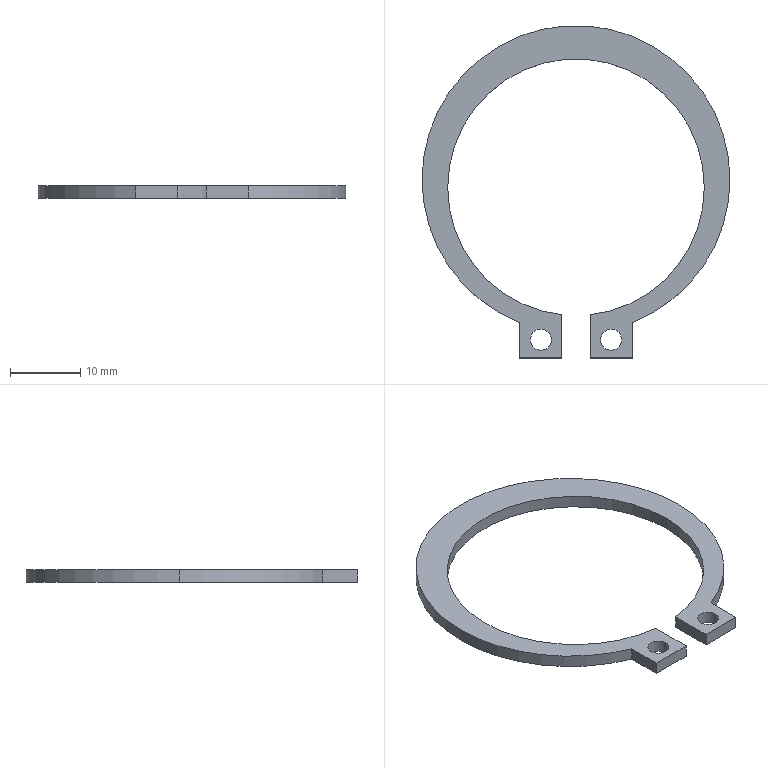Part | STEP file | Mkt stator clip | 1 solid | 18 faces | box 43.8 x 47.287 x 1.8 mm | volume 874.267 mm3 | cylinder 10 | plane 8 | commonest cylinder face diameters 3 x4 36.5 x3 43.8 x3
STEP:
#1=CARTESIAN_POINT('',(0.,0.,0.));
#2=DIRECTION('',(0.,0.,1.));
#3=DIRECTION('',(1.,0.,0.));
#4=AXIS2_PLACEMENT_3D('',#1,#2,#3);
#5=CARTESIAN_POINT('',(3.5,-21.7,1.8));
#6=VERTEX_POINT('',#5);
#7=CARTESIAN_POINT('',(3.5,-21.7,0.));
#8=VERTEX_POINT('',#7);
#9=CARTESIAN_POINT('',(3.5,-21.7,1.8));
#10=DIRECTION('',(0.,0.,-1.));
#11=VECTOR('',#10,1.);
#12=LINE('',#9,#11);
#13=CARTESIAN_POINT('',(5.,-21.7,1.8));
#14=DIRECTION('',(0.,0.,-1.));
#15=DIRECTION('',(-1.,0.,0.));
#16=AXIS2_PLACEMENT_3D('',#13,#14,#15);
#17=CYLINDRICAL_SURFACE('',#16,1.5);
#18=CARTESIAN_POINT('',(6.283,0.));
#19=DIRECTION('',(0.,1.));
#20=VECTOR('',#19,1.);
#21=LINE('',#18,#20);
#22=(GEOMETRIC_REPRESENTATION_CONTEXT(2)PARAMETRIC_REPRESENTATION_CONTEXT()REPRESENTATION_CONTEXT('',''));
#23=DEFINITIONAL_REPRESENTATION('',(#21),#22);
#24=PCURVE('',#17,#23);
#25=CARTESIAN_POINT('',(5.,-21.7,1.8));
#26=DIRECTION('',(0.,0.,-1.));
#27=DIRECTION('',(-1.,0.,0.));
#28=AXIS2_PLACEMENT_3D('',#25,#26,#27);
#29=CYLINDRICAL_SURFACE('',#28,1.5);
#30=CARTESIAN_POINT('',(0.,0.));
#31=DIRECTION('',(0.,1.));
#32=VECTOR('',#31,1.);
#33=LINE('',#30,#32);
#34=(GEOMETRIC_REPRESENTATION_CONTEXT(2)PARAMETRIC_REPRESENTATION_CONTEXT()REPRESENTATION_CONTEXT('',''));
#35=DEFINITIONAL_REPRESENTATION('',(#33),#34);
#36=PCURVE('',#29,#35);
#37=SURFACE_CURVE('',#12,(#24,#36),.PCURVE_S1.);
#38=EDGE_CURVE('',#6,#8,#37,.T.);
#39=ORIENTED_EDGE('',*,*,#38,.T.);
#40=CARTESIAN_POINT('',(6.5,-21.7,0.));
#41=VERTEX_POINT('',#40);
#42=CARTESIAN_POINT('',(5.,-21.7,0.));
#43=DIRECTION('',(0.,0.,1.));
#44=DIRECTION('',(-1.,0.,0.));
#45=AXIS2_PLACEMENT_3D('',#42,#43,#44);
#46=CIRCLE('',#45,1.5);
#47=CARTESIAN_POINT('',(6.283,1.8));
#48=DIRECTION('',(-1.,0.));
#49=VECTOR('',#48,1.);
#50=LINE('',#47,#49);
#51=(GEOMETRIC_REPRESENTATION_CONTEXT(2)PARAMETRIC_REPRESENTATION_CONTEXT()REPRESENTATION_CONTEXT('',''));
#52=DEFINITIONAL_REPRESENTATION('',(#50),#51);
#53=PCURVE('',#17,#52);
#54=CARTESIAN_POINT('',(0.,0.,0.));
#55=DIRECTION('',(0.,0.,1.));
#56=DIRECTION('',(1.,0.,0.));
#57=AXIS2_PLACEMENT_3D('',#54,#55,#56);
#58=PLANE('',#57);
#59=CARTESIAN_POINT('',(5.,-21.7));
#60=DIRECTION('',(-1.,0.));
#61=AXIS2_PLACEMENT_2D('',#59,#60);
#62=CIRCLE('',#61,1.5);
#63=(GEOMETRIC_REPRESENTATION_CONTEXT(2)PARAMETRIC_REPRESENTATION_CONTEXT()REPRESENTATION_CONTEXT('',''));
#64=DEFINITIONAL_REPRESENTATION('',(#62),#63);
#65=PCURVE('',#58,#64);
#66=SURFACE_CURVE('',#46,(#53,#65),.PCURVE_S1.);
#67=EDGE_CURVE('',#8,#41,#66,.T.);
#68=ORIENTED_EDGE('',*,*,#67,.T.);
#69=CARTESIAN_POINT('',(6.5,-21.7,1.8));
#70=VERTEX_POINT('',#69);
#71=CARTESIAN_POINT('',(6.5,-21.7,1.8));
#72=DIRECTION('',(0.,0.,-1.));
#73=VECTOR('',#72,1.);
#74=LINE('',#71,#73);
#75=CARTESIAN_POINT('',(3.142,0.));
#76=DIRECTION('',(0.,1.));
#77=VECTOR('',#76,1.);
#78=LINE('',#75,#77);
#79=(GEOMETRIC_REPRESENTATION_CONTEXT(2)PARAMETRIC_REPRESENTATION_CONTEXT()REPRESENTATION_CONTEXT('',''));
#80=DEFINITIONAL_REPRESENTATION('',(#78),#79);
#81=PCURVE('',#17,#80);
#82=CARTESIAN_POINT('',(3.142,0.));
#83=DIRECTION('',(0.,1.));
#84=VECTOR('',#83,1.);
#85=LINE('',#82,#84);
#86=(GEOMETRIC_REPRESENTATION_CONTEXT(2)PARAMETRIC_REPRESENTATION_CONTEXT()REPRESENTATION_CONTEXT('',''));
#87=DEFINITIONAL_REPRESENTATION('',(#85),#86);
#88=PCURVE('',#29,#87);
#89=SURFACE_CURVE('',#74,(#81,#88),.PCURVE_S1.);
#90=EDGE_CURVE('',#70,#41,#89,.T.);
#91=ORIENTED_EDGE('',*,*,#90,.F.);
#92=CARTESIAN_POINT('',(5.,-21.7,1.8));
#93=DIRECTION('',(0.,0.,-1.));
#94=DIRECTION('',(-1.,0.,0.));
#95=AXIS2_PLACEMENT_3D('',#92,#93,#94);
#96=CIRCLE('',#95,1.5);
#97=CARTESIAN_POINT('',(0.,0.));
#98=DIRECTION('',(1.,0.));
#99=VECTOR('',#98,1.);
#100=LINE('',#97,#99);
#101=(GEOMETRIC_REPRESENTATION_CONTEXT(2)PARAMETRIC_REPRESENTATION_CONTEXT()REPRESENTATION_CONTEXT('',''));
#102=DEFINITIONAL_REPRESENTATION('',(#100),#101);
#103=PCURVE('',#17,#102);
#104=CARTESIAN_POINT('',(0.,0.,1.8));
#105=DIRECTION('',(0.,0.,1.));
#106=DIRECTION('',(1.,0.,0.));
#107=AXIS2_PLACEMENT_3D('',#104,#105,#106);
#108=PLANE('',#107);
#109=CARTESIAN_POINT('',(3.5,-21.7));
#110=CARTESIAN_POINT('',(3.5,-19.102));
#111=CARTESIAN_POINT('',(5.75,-20.401));
#112=CARTESIAN_POINT('',(8.,-21.7));
#113=CARTESIAN_POINT('',(5.75,-22.999));
#114=CARTESIAN_POINT('',(3.5,-24.298));
#115=CARTESIAN_POINT('',(3.5,-21.7));
#116=(BOUNDED_CURVE()B_SPLINE_CURVE(2,(#109,#110,#111,#112,#113,#114,#115),.UNSPECIFIED.,.T.,.F.)B_SPLINE_CURVE_WITH_KNOTS((1,2,2,2,2,1),(-2.094,0.,2.094,4.189,6.283,8.378),.UNSPECIFIED.)CURVE()GEOMETRIC_REPRESENTATION_ITEM()RATIONAL_B_SPLINE_CURVE((1.,0.5,1.,0.5,1.,0.5,1.))REPRESENTATION_ITEM(''));
#117=(GEOMETRIC_REPRESENTATION_CONTEXT(2)PARAMETRIC_REPRESENTATION_CONTEXT()REPRESENTATION_CONTEXT('',''));
#118=DEFINITIONAL_REPRESENTATION('',(#116),#117);
#119=PCURVE('',#108,#118);
#120=SURFACE_CURVE('',#96,(#103,#119),.PCURVE_S1.);
#121=EDGE_CURVE('',#70,#6,#120,.T.);
#122=ORIENTED_EDGE('',*,*,#121,.T.);
#123=EDGE_LOOP('',(#39,#68,#91,#122));
#124=FACE_BOUND('',#123,.F.);
#125=ADVANCED_FACE('',(#124),#17,.F.);
#126=CARTESIAN_POINT('',(21.9,1.1,1.8));
#127=VERTEX_POINT('',#126);
#128=CARTESIAN_POINT('',(-21.9,1.1,1.8));
#129=VERTEX_POINT('',#128);
#130=CARTESIAN_POINT('',(0.,1.1,1.8));
#131=DIRECTION('',(0.,0.,1.));
#132=DIRECTION('',(-1.,0.,0.));
#133=AXIS2_PLACEMENT_3D('',#130,#131,#132);
#134=CIRCLE('',#133,21.9);
#135=CARTESIAN_POINT('',(0.,1.1,1.8));
#136=DIRECTION('',(0.,0.,-1.));
#137=DIRECTION('',(-1.,0.,0.));
#138=AXIS2_PLACEMENT_3D('',#135,#136,#137);
#139=CYLINDRICAL_SURFACE('',#138,21.9);
#140=CARTESIAN_POINT('',(6.283,0.));
#141=DIRECTION('',(-1.,0.));
#142=VECTOR('',#141,1.);
#143=LINE('',#140,#142);
#144=(GEOMETRIC_REPRESENTATION_CONTEXT(2)PARAMETRIC_REPRESENTATION_CONTEXT()REPRESENTATION_CONTEXT('',''));
#145=DEFINITIONAL_REPRESENTATION('',(#143),#144);
#146=PCURVE('',#139,#145);
#147=CARTESIAN_POINT('',(0.,1.1));
#148=DIRECTION('',(-1.,0.));
#149=AXIS2_PLACEMENT_2D('',#147,#148);
#150=CIRCLE('',#149,21.9);
#151=(GEOMETRIC_REPRESENTATION_CONTEXT(2)PARAMETRIC_REPRESENTATION_CONTEXT()REPRESENTATION_CONTEXT('',''));
#152=DEFINITIONAL_REPRESENTATION('',(#150),#151);
#153=PCURVE('',#108,#152);
#154=SURFACE_CURVE('',#134,(#146,#153),.PCURVE_S1.);
#155=EDGE_CURVE('',#127,#129,#154,.T.);
#156=ORIENTED_EDGE('',*,*,#155,.F.);
#157=CARTESIAN_POINT('',(21.9,1.1,0.));
#158=VERTEX_POINT('',#157);
#159=CARTESIAN_POINT('',(21.9,1.1,1.8));
#160=DIRECTION('',(0.,0.,-1.));
#161=VECTOR('',#160,1.);
#162=LINE('',#159,#161);
#163=CARTESIAN_POINT('',(3.142,0.));
#164=DIRECTION('',(0.,1.));
#165=VECTOR('',#164,1.);
#166=LINE('',#163,#165);
#167=(GEOMETRIC_REPRESENTATION_CONTEXT(2)PARAMETRIC_REPRESENTATION_CONTEXT()REPRESENTATION_CONTEXT('',''));
#168=DEFINITIONAL_REPRESENTATION('',(#166),#167);
#169=PCURVE('',#139,#168);
#170=CARTESIAN_POINT('',(0.,1.1,1.8));
#171=DIRECTION('',(0.,0.,-1.));
#172=DIRECTION('',(-1.,0.,0.));
#173=AXIS2_PLACEMENT_3D('',#170,#171,#172);
#174=CYLINDRICAL_SURFACE('',#173,21.9);
#175=CARTESIAN_POINT('',(3.142,0.));
#176=DIRECTION('',(0.,1.));
#177=VECTOR('',#176,1.);
#178=LINE('',#175,#177);
#179=(GEOMETRIC_REPRESENTATION_CONTEXT(2)PARAMETRIC_REPRESENTATION_CONTEXT()REPRESENTATION_CONTEXT('',''));
#180=DEFINITIONAL_REPRESENTATION('',(#178),#179);
#181=PCURVE('',#174,#180);
#182=SURFACE_CURVE('',#162,(#169,#181),.PCURVE_S1.);
#183=EDGE_CURVE('',#127,#158,#182,.T.);
#184=ORIENTED_EDGE('',*,*,#183,.T.);
#185=CARTESIAN_POINT('',(-21.9,1.1,0.));
#186=VERTEX_POINT('',#185);
#187=CARTESIAN_POINT('',(0.,1.1,0.));
#188=DIRECTION('',(0.,0.,1.));
#189=DIRECTION('',(-1.,0.,0.));
#190=AXIS2_PLACEMENT_3D('',#187,#188,#189);
#191=CIRCLE('',#190,21.9);
#192=CARTESIAN_POINT('',(6.283,1.8));
#193=DIRECTION('',(-1.,0.));
#194=VECTOR('',#193,1.);
#195=LINE('',#192,#194);
#196=(GEOMETRIC_REPRESENTATION_CONTEXT(2)PARAMETRIC_REPRESENTATION_CONTEXT()REPRESENTATION_CONTEXT('',''));
#197=DEFINITIONAL_REPRESENTATION('',(#195),#196);
#198=PCURVE('',#139,#197);
#199=CARTESIAN_POINT('',(0.,1.1));
#200=DIRECTION('',(-1.,0.));
#201=AXIS2_PLACEMENT_2D('',#199,#200);
#202=CIRCLE('',#201,21.9);
#203=(GEOMETRIC_REPRESENTATION_CONTEXT(2)PARAMETRIC_REPRESENTATION_CONTEXT()REPRESENTATION_CONTEXT('',''));
#204=DEFINITIONAL_REPRESENTATION('',(#202),#203);
#205=PCURVE('',#58,#204);
#206=SURFACE_CURVE('',#191,(#198,#205),.PCURVE_S1.);
#207=EDGE_CURVE('',#158,#186,#206,.T.);
#208=ORIENTED_EDGE('',*,*,#207,.T.);
#209=CARTESIAN_POINT('',(-21.9,1.1,1.8));
#210=DIRECTION('',(0.,0.,-1.));
#211=VECTOR('',#210,1.);
#212=LINE('',#209,#211);
#213=CARTESIAN_POINT('',(0.,0.));
#214=DIRECTION('',(0.,1.));
#215=VECTOR('',#214,1.);
#216=LINE('',#213,#215);
#217=(GEOMETRIC_REPRESENTATION_CONTEXT(2)PARAMETRIC_REPRESENTATION_CONTEXT()REPRESENTATION_CONTEXT('',''));
#218=DEFINITIONAL_REPRESENTATION('',(#216),#217);
#219=PCURVE('',#139,#218);
#220=CARTESIAN_POINT('',(0.,1.1,1.8));
#221=DIRECTION('',(0.,0.,-1.));
#222=DIRECTION('',(-1.,0.,0.));
#223=AXIS2_PLACEMENT_3D('',#220,#221,#222);
#224=CYLINDRICAL_SURFACE('',#223,21.9);
#225=CARTESIAN_POINT('',(6.283,0.));
#226=DIRECTION('',(0.,1.));
#227=VECTOR('',#226,1.);
#228=LINE('',#225,#227);
#229=(GEOMETRIC_REPRESENTATION_CONTEXT(2)PARAMETRIC_REPRESENTATION_CONTEXT()REPRESENTATION_CONTEXT('',''));
#230=DEFINITIONAL_REPRESENTATION('',(#228),#229);
#231=PCURVE('',#224,#230);
#232=SURFACE_CURVE('',#212,(#219,#231),.PCURVE_S1.);
#233=EDGE_CURVE('',#129,#186,#232,.T.);
#234=ORIENTED_EDGE('',*,*,#233,.F.);
#235=EDGE_LOOP('',(#156,#184,#208,#234));
#236=FACE_BOUND('',#235,.T.);
#237=ADVANCED_FACE('',(#236),#139,.T.);
#238=CARTESIAN_POINT('',(-8.,-19.287,1.8));
#239=VERTEX_POINT('',#238);
#240=CARTESIAN_POINT('',(0.,1.1,1.8));
#241=DIRECTION('',(0.,0.,1.));
#242=DIRECTION('',(-1.,0.,0.));
#243=AXIS2_PLACEMENT_3D('',#240,#241,#242);
#244=CIRCLE('',#243,21.9);
#245=CARTESIAN_POINT('',(6.283,0.));
#246=DIRECTION('',(-1.,0.));
#247=VECTOR('',#246,1.);
#248=LINE('',#245,#247);
#249=(GEOMETRIC_REPRESENTATION_CONTEXT(2)PARAMETRIC_REPRESENTATION_CONTEXT()REPRESENTATION_CONTEXT('',''));
#250=DEFINITIONAL_REPRESENTATION('',(#248),#249);
#251=PCURVE('',#224,#250);
#252=CARTESIAN_POINT('',(0.,1.1));
#253=DIRECTION('',(-1.,0.));
#254=AXIS2_PLACEMENT_2D('',#252,#253);
#255=CIRCLE('',#254,21.9);
#256=(GEOMETRIC_REPRESENTATION_CONTEXT(2)PARAMETRIC_REPRESENTATION_CONTEXT()REPRESENTATION_CONTEXT('',''));
#257=DEFINITIONAL_REPRESENTATION('',(#255),#256);
#258=PCURVE('',#108,#257);
#259=SURFACE_CURVE('',#244,(#251,#258),.PCURVE_S1.);
#260=EDGE_CURVE('',#129,#239,#259,.T.);
#261=ORIENTED_EDGE('',*,*,#260,.F.);
#262=ORIENTED_EDGE('',*,*,#233,.T.);
#263=CARTESIAN_POINT('',(-8.,-19.287,0.));
#264=VERTEX_POINT('',#263);
#265=CARTESIAN_POINT('',(0.,1.1,0.));
#266=DIRECTION('',(0.,0.,1.));
#267=DIRECTION('',(-1.,0.,0.));
#268=AXIS2_PLACEMENT_3D('',#265,#266,#267);
#269=CIRCLE('',#268,21.9);
#270=CARTESIAN_POINT('',(6.283,1.8));
#271=DIRECTION('',(-1.,0.));
#272=VECTOR('',#271,1.);
#273=LINE('',#270,#272);
#274=(GEOMETRIC_REPRESENTATION_CONTEXT(2)PARAMETRIC_REPRESENTATION_CONTEXT()REPRESENTATION_CONTEXT('',''));
#275=DEFINITIONAL_REPRESENTATION('',(#273),#274);
#276=PCURVE('',#224,#275);
#277=CARTESIAN_POINT('',(0.,1.1));
#278=DIRECTION('',(-1.,0.));
#279=AXIS2_PLACEMENT_2D('',#277,#278);
#280=CIRCLE('',#279,21.9);
#281=(GEOMETRIC_REPRESENTATION_CONTEXT(2)PARAMETRIC_REPRESENTATION_CONTEXT()REPRESENTATION_CONTEXT('',''));
#282=DEFINITIONAL_REPRESENTATION('',(#280),#281);
#283=PCURVE('',#58,#282);
#284=SURFACE_CURVE('',#269,(#276,#283),.PCURVE_S1.);
#285=EDGE_CURVE('',#186,#264,#284,.T.);
#286=ORIENTED_EDGE('',*,*,#285,.T.);
#287=CARTESIAN_POINT('',(-8.,-19.287,1.8));
#288=DIRECTION('',(0.,0.,1.));
#289=VECTOR('',#288,1.);
#290=LINE('',#287,#289);
#291=CARTESIAN_POINT('',(5.086,0.));
#292=DIRECTION('',(0.,-1.));
#293=VECTOR('',#292,1.);
#294=LINE('',#291,#293);
#295=(GEOMETRIC_REPRESENTATION_CONTEXT(2)PARAMETRIC_REPRESENTATION_CONTEXT()REPRESENTATION_CONTEXT('',''));
#296=DEFINITIONAL_REPRESENTATION('',(#294),#295);
#297=PCURVE('',#224,#296);
#298=CARTESIAN_POINT('',(-8.,-24.287,1.8));
#299=DIRECTION('',(1.,0.,0.));
#300=DIRECTION('',(0.,1.,0.));
#301=AXIS2_PLACEMENT_3D('',#298,#299,#300);
#302=PLANE('',#301);
#303=CARTESIAN_POINT('',(5.,0.));
#304=DIRECTION('',(0.,1.));
#305=VECTOR('',#304,1.);
#306=LINE('',#303,#305);
#307=(GEOMETRIC_REPRESENTATION_CONTEXT(2)PARAMETRIC_REPRESENTATION_CONTEXT()REPRESENTATION_CONTEXT('',''));
#308=DEFINITIONAL_REPRESENTATION('',(#306),#307);
#309=PCURVE('',#302,#308);
#310=SURFACE_CURVE('',#290,(#297,#309),.PCURVE_S1.);
#311=EDGE_CURVE('',#264,#239,#310,.T.);
#312=ORIENTED_EDGE('',*,*,#311,.T.);
#313=EDGE_LOOP('',(#261,#262,#286,#312));
#314=FACE_BOUND('',#313,.T.);
#315=ADVANCED_FACE('',(#314),#224,.T.);
#316=CARTESIAN_POINT('',(2.,-18.14,0.));
#317=VERTEX_POINT('',#316);
#318=CARTESIAN_POINT('',(2.,-18.14,1.8));
#319=VERTEX_POINT('',#318);
#320=CARTESIAN_POINT('',(2.,-18.14,1.8));
#321=DIRECTION('',(0.,0.,1.));
#322=VECTOR('',#321,1.);
#323=LINE('',#320,#322);
#324=CARTESIAN_POINT('',(0.,0.,1.8));
#325=DIRECTION('',(0.,0.,-1.));
#326=DIRECTION('',(-1.,0.,0.));
#327=AXIS2_PLACEMENT_3D('',#324,#325,#326);
#328=CYLINDRICAL_SURFACE('',#327,18.25);
#329=CARTESIAN_POINT('',(4.603,0.));
#330=DIRECTION('',(0.,-1.));
#331=VECTOR('',#330,1.);
#332=LINE('',#329,#331);
#333=(GEOMETRIC_REPRESENTATION_CONTEXT(2)PARAMETRIC_REPRESENTATION_CONTEXT()REPRESENTATION_CONTEXT('',''));
#334=DEFINITIONAL_REPRESENTATION('',(#332),#333);
#335=PCURVE('',#328,#334);
#336=CARTESIAN_POINT('',(2.,-24.287,1.8));
#337=DIRECTION('',(1.,0.,0.));
#338=DIRECTION('',(0.,1.,0.));
#339=AXIS2_PLACEMENT_3D('',#336,#337,#338);
#340=PLANE('',#339);
#341=CARTESIAN_POINT('',(6.146,0.));
#342=DIRECTION('',(0.,1.));
#343=VECTOR('',#342,1.);
#344=LINE('',#341,#343);
#345=(GEOMETRIC_REPRESENTATION_CONTEXT(2)PARAMETRIC_REPRESENTATION_CONTEXT()REPRESENTATION_CONTEXT('',''));
#346=DEFINITIONAL_REPRESENTATION('',(#344),#345);
#347=PCURVE('',#340,#346);
#348=SURFACE_CURVE('',#323,(#335,#347),.PCURVE_S1.);
#349=EDGE_CURVE('',#317,#319,#348,.T.);
#350=ORIENTED_EDGE('',*,*,#349,.F.);
#351=CARTESIAN_POINT('',(18.25,0.,0.));
#352=VERTEX_POINT('',#351);
#353=CARTESIAN_POINT('',(0.,0.,0.));
#354=DIRECTION('',(0.,0.,1.));
#355=DIRECTION('',(-1.,0.,0.));
#356=AXIS2_PLACEMENT_3D('',#353,#354,#355);
#357=CIRCLE('',#356,18.25);
#358=CARTESIAN_POINT('',(6.283,1.8));
#359=DIRECTION('',(-1.,0.));
#360=VECTOR('',#359,1.);
#361=LINE('',#358,#360);
#362=(GEOMETRIC_REPRESENTATION_CONTEXT(2)PARAMETRIC_REPRESENTATION_CONTEXT()REPRESENTATION_CONTEXT('',''));
#363=DEFINITIONAL_REPRESENTATION('',(#361),#362);
#364=PCURVE('',#328,#363);
#365=CARTESIAN_POINT('',(0.,0.));
#366=DIRECTION('',(-1.,0.));
#367=AXIS2_PLACEMENT_2D('',#365,#366);
#368=CIRCLE('',#367,18.25);
#369=(GEOMETRIC_REPRESENTATION_CONTEXT(2)PARAMETRIC_REPRESENTATION_CONTEXT()REPRESENTATION_CONTEXT('',''));
#370=DEFINITIONAL_REPRESENTATION('',(#368),#369);
#371=PCURVE('',#58,#370);
#372=SURFACE_CURVE('',#357,(#364,#371),.PCURVE_S1.);
#373=EDGE_CURVE('',#317,#352,#372,.T.);
#374=ORIENTED_EDGE('',*,*,#373,.T.);
#375=CARTESIAN_POINT('',(18.25,0.,1.8));
#376=VERTEX_POINT('',#375);
#377=CARTESIAN_POINT('',(18.25,0.,1.8));
#378=DIRECTION('',(0.,0.,-1.));
#379=VECTOR('',#378,1.);
#380=LINE('',#377,#379);
#381=CARTESIAN_POINT('',(3.142,0.));
#382=DIRECTION('',(0.,1.));
#383=VECTOR('',#382,1.);
#384=LINE('',#381,#383);
#385=(GEOMETRIC_REPRESENTATION_CONTEXT(2)PARAMETRIC_REPRESENTATION_CONTEXT()REPRESENTATION_CONTEXT('',''));
#386=DEFINITIONAL_REPRESENTATION('',(#384),#385);
#387=PCURVE('',#328,#386);
#388=CARTESIAN_POINT('',(0.,0.,1.8));
#389=DIRECTION('',(0.,0.,-1.));
#390=DIRECTION('',(-1.,0.,0.));
#391=AXIS2_PLACEMENT_3D('',#388,#389,#390);
#392=CYLINDRICAL_SURFACE('',#391,18.25);
#393=CARTESIAN_POINT('',(3.142,0.));
#394=DIRECTION('',(0.,1.));
#395=VECTOR('',#394,1.);
#396=LINE('',#393,#395);
#397=(GEOMETRIC_REPRESENTATION_CONTEXT(2)PARAMETRIC_REPRESENTATION_CONTEXT()REPRESENTATION_CONTEXT('',''));
#398=DEFINITIONAL_REPRESENTATION('',(#396),#397);
#399=PCURVE('',#392,#398);
#400=SURFACE_CURVE('',#380,(#387,#399),.PCURVE_S1.);
#401=EDGE_CURVE('',#376,#352,#400,.T.);
#402=ORIENTED_EDGE('',*,*,#401,.F.);
#403=CARTESIAN_POINT('',(0.,0.,1.8));
#404=DIRECTION('',(0.,0.,-1.));
#405=DIRECTION('',(-1.,0.,0.));
#406=AXIS2_PLACEMENT_3D('',#403,#404,#405);
#407=CIRCLE('',#406,18.25);
#408=CARTESIAN_POINT('',(0.,0.));
#409=DIRECTION('',(1.,0.));
#410=VECTOR('',#409,1.);
#411=LINE('',#408,#410);
#412=(GEOMETRIC_REPRESENTATION_CONTEXT(2)PARAMETRIC_REPRESENTATION_CONTEXT()REPRESENTATION_CONTEXT('',''));
#413=DEFINITIONAL_REPRESENTATION('',(#411),#412);
#414=PCURVE('',#328,#413);
#415=CARTESIAN_POINT('',(-18.25,0.));
#416=CARTESIAN_POINT('',(-18.25,31.61));
#417=CARTESIAN_POINT('',(9.125,15.805));
#418=CARTESIAN_POINT('',(36.5,0.));
#419=CARTESIAN_POINT('',(9.125,-15.805));
#420=CARTESIAN_POINT('',(-18.25,-31.61));
#421=CARTESIAN_POINT('',(-18.25,0.));
#422=(BOUNDED_CURVE()B_SPLINE_CURVE(2,(#415,#416,#417,#418,#419,#420,#421),.UNSPECIFIED.,.T.,.F.)B_SPLINE_CURVE_WITH_KNOTS((1,2,2,2,2,1),(-2.094,0.,2.094,4.189,6.283,8.378),.UNSPECIFIED.)CURVE()GEOMETRIC_REPRESENTATION_ITEM()RATIONAL_B_SPLINE_CURVE((1.,0.5,1.,0.5,1.,0.5,1.))REPRESENTATION_ITEM(''));
#423=(GEOMETRIC_REPRESENTATION_CONTEXT(2)PARAMETRIC_REPRESENTATION_CONTEXT()REPRESENTATION_CONTEXT('',''));
#424=DEFINITIONAL_REPRESENTATION('',(#422),#423);
#425=PCURVE('',#108,#424);
#426=SURFACE_CURVE('',#407,(#414,#425),.PCURVE_S1.);
#427=EDGE_CURVE('',#376,#319,#426,.T.);
#428=ORIENTED_EDGE('',*,*,#427,.T.);
#429=EDGE_LOOP('',(#350,#374,#402,#428));
#430=FACE_BOUND('',#429,.F.);
#431=ADVANCED_FACE('',(#430),#328,.F.);
#432=CARTESIAN_POINT('',(-18.25,0.,0.));
#433=VERTEX_POINT('',#432);
#434=CARTESIAN_POINT('',(0.,0.,0.));
#435=DIRECTION('',(0.,0.,1.));
#436=DIRECTION('',(-1.,0.,0.));
#437=AXIS2_PLACEMENT_3D('',#434,#435,#436);
#438=CIRCLE('',#437,18.25);
#439=CARTESIAN_POINT('',(6.283,1.8));
#440=DIRECTION('',(-1.,0.));
#441=VECTOR('',#440,1.);
#442=LINE('',#439,#441);
#443=(GEOMETRIC_REPRESENTATION_CONTEXT(2)PARAMETRIC_REPRESENTATION_CONTEXT()REPRESENTATION_CONTEXT('',''));
#444=DEFINITIONAL_REPRESENTATION('',(#442),#443);
#445=PCURVE('',#392,#444);
#446=CARTESIAN_POINT('',(0.,0.));
#447=DIRECTION('',(-1.,0.));
#448=AXIS2_PLACEMENT_2D('',#446,#447);
#449=CIRCLE('',#448,18.25);
#450=(GEOMETRIC_REPRESENTATION_CONTEXT(2)PARAMETRIC_REPRESENTATION_CONTEXT()REPRESENTATION_CONTEXT('',''));
#451=DEFINITIONAL_REPRESENTATION('',(#449),#450);
#452=PCURVE('',#58,#451);
#453=SURFACE_CURVE('',#438,(#445,#452),.PCURVE_S1.);
#454=EDGE_CURVE('',#352,#433,#453,.T.);
#455=ORIENTED_EDGE('',*,*,#454,.T.);
#456=CARTESIAN_POINT('',(-18.25,0.,1.8));
#457=VERTEX_POINT('',#456);
#458=CARTESIAN_POINT('',(-18.25,0.,1.8));
#459=DIRECTION('',(0.,0.,-1.));
#460=VECTOR('',#459,1.);
#461=LINE('',#458,#460);
#462=CARTESIAN_POINT('',(0.,0.));
#463=DIRECTION('',(0.,1.));
#464=VECTOR('',#463,1.);
#465=LINE('',#462,#464);
#466=(GEOMETRIC_REPRESENTATION_CONTEXT(2)PARAMETRIC_REPRESENTATION_CONTEXT()REPRESENTATION_CONTEXT('',''));
#467=DEFINITIONAL_REPRESENTATION('',(#465),#466);
#468=PCURVE('',#392,#467);
#469=CARTESIAN_POINT('',(0.,0.,1.8));
#470=DIRECTION('',(0.,0.,-1.));
#471=DIRECTION('',(-1.,0.,0.));
#472=AXIS2_PLACEMENT_3D('',#469,#470,#471);
#473=CYLINDRICAL_SURFACE('',#472,18.25);
#474=CARTESIAN_POINT('',(6.283,0.));
#475=DIRECTION('',(0.,1.));
#476=VECTOR('',#475,1.);
#477=LINE('',#474,#476);
#478=(GEOMETRIC_REPRESENTATION_CONTEXT(2)PARAMETRIC_REPRESENTATION_CONTEXT()REPRESENTATION_CONTEXT('',''));
#479=DEFINITIONAL_REPRESENTATION('',(#477),#478);
#480=PCURVE('',#473,#479);
#481=SURFACE_CURVE('',#461,(#468,#480),.PCURVE_S1.);
#482=EDGE_CURVE('',#457,#433,#481,.T.);
#483=ORIENTED_EDGE('',*,*,#482,.F.);
#484=CARTESIAN_POINT('',(0.,0.,1.8));
#485=DIRECTION('',(0.,0.,-1.));
#486=DIRECTION('',(-1.,0.,0.));
#487=AXIS2_PLACEMENT_3D('',#484,#485,#486);
#488=CIRCLE('',#487,18.25);
#489=CARTESIAN_POINT('',(0.,0.));
#490=DIRECTION('',(1.,0.));
#491=VECTOR('',#490,1.);
#492=LINE('',#489,#491);
#493=(GEOMETRIC_REPRESENTATION_CONTEXT(2)PARAMETRIC_REPRESENTATION_CONTEXT()REPRESENTATION_CONTEXT('',''));
#494=DEFINITIONAL_REPRESENTATION('',(#492),#493);
#495=PCURVE('',#392,#494);
#496=CARTESIAN_POINT('',(-18.25,0.));
#497=CARTESIAN_POINT('',(-18.25,31.61));
#498=CARTESIAN_POINT('',(9.125,15.805));
#499=CARTESIAN_POINT('',(36.5,0.));
#500=CARTESIAN_POINT('',(9.125,-15.805));
#501=CARTESIAN_POINT('',(-18.25,-31.61));
#502=CARTESIAN_POINT('',(-18.25,0.));
#503=(BOUNDED_CURVE()B_SPLINE_CURVE(2,(#496,#497,#498,#499,#500,#501,#502),.UNSPECIFIED.,.T.,.F.)B_SPLINE_CURVE_WITH_KNOTS((1,2,2,2,2,1),(-2.094,0.,2.094,4.189,6.283,8.378),.UNSPECIFIED.)CURVE()GEOMETRIC_REPRESENTATION_ITEM()RATIONAL_B_SPLINE_CURVE((1.,0.5,1.,0.5,1.,0.5,1.))REPRESENTATION_ITEM(''));
#504=(GEOMETRIC_REPRESENTATION_CONTEXT(2)PARAMETRIC_REPRESENTATION_CONTEXT()REPRESENTATION_CONTEXT('',''));
#505=DEFINITIONAL_REPRESENTATION('',(#503),#504);
#506=PCURVE('',#108,#505);
#507=SURFACE_CURVE('',#488,(#495,#506),.PCURVE_S1.);
#508=EDGE_CURVE('',#457,#376,#507,.T.);
#509=ORIENTED_EDGE('',*,*,#508,.T.);
#510=ORIENTED_EDGE('',*,*,#401,.T.);
#511=EDGE_LOOP('',(#455,#483,#509,#510));
#512=FACE_BOUND('',#511,.F.);
#513=ADVANCED_FACE('',(#512),#392,.F.);
#514=CARTESIAN_POINT('',(-6.5,-21.7,1.8));
#515=VERTEX_POINT('',#514);
#516=CARTESIAN_POINT('',(-6.5,-21.7,0.));
#517=VERTEX_POINT('',#516);
#518=CARTESIAN_POINT('',(-6.5,-21.7,1.8));
#519=DIRECTION('',(0.,0.,-1.));
#520=VECTOR('',#519,1.);
#521=LINE('',#518,#520);
#522=CARTESIAN_POINT('',(-5.,-21.7,1.8));
#523=DIRECTION('',(0.,0.,-1.));
#524=DIRECTION('',(-1.,0.,0.));
#525=AXIS2_PLACEMENT_3D('',#522,#523,#524);
#526=CYLINDRICAL_SURFACE('',#525,1.5);
#527=CARTESIAN_POINT('',(6.283,0.));
#528=DIRECTION('',(0.,1.));
#529=VECTOR('',#528,1.);
#530=LINE('',#527,#529);
#531=(GEOMETRIC_REPRESENTATION_CONTEXT(2)PARAMETRIC_REPRESENTATION_CONTEXT()REPRESENTATION_CONTEXT('',''));
#532=DEFINITIONAL_REPRESENTATION('',(#530),#531);
#533=PCURVE('',#526,#532);
#534=CARTESIAN_POINT('',(-5.,-21.7,1.8));
#535=DIRECTION('',(0.,0.,-1.));
#536=DIRECTION('',(-1.,0.,0.));
#537=AXIS2_PLACEMENT_3D('',#534,#535,#536);
#538=CYLINDRICAL_SURFACE('',#537,1.5);
#539=CARTESIAN_POINT('',(0.,0.));
#540=DIRECTION('',(0.,1.));
#541=VECTOR('',#540,1.);
#542=LINE('',#539,#541);
#543=(GEOMETRIC_REPRESENTATION_CONTEXT(2)PARAMETRIC_REPRESENTATION_CONTEXT()REPRESENTATION_CONTEXT('',''));
#544=DEFINITIONAL_REPRESENTATION('',(#542),#543);
#545=PCURVE('',#538,#544);
#546=SURFACE_CURVE('',#521,(#533,#545),.PCURVE_S1.);
#547=EDGE_CURVE('',#515,#517,#546,.T.);
#548=ORIENTED_EDGE('',*,*,#547,.T.);
#549=CARTESIAN_POINT('',(-3.5,-21.7,0.));
#550=VERTEX_POINT('',#549);
#551=CARTESIAN_POINT('',(-5.,-21.7,0.));
#552=DIRECTION('',(0.,0.,1.));
#553=DIRECTION('',(-1.,0.,0.));
#554=AXIS2_PLACEMENT_3D('',#551,#552,#553);
#555=CIRCLE('',#554,1.5);
#556=CARTESIAN_POINT('',(6.283,1.8));
#557=DIRECTION('',(-1.,0.));
#558=VECTOR('',#557,1.);
#559=LINE('',#556,#558);
#560=(GEOMETRIC_REPRESENTATION_CONTEXT(2)PARAMETRIC_REPRESENTATION_CONTEXT()REPRESENTATION_CONTEXT('',''));
#561=DEFINITIONAL_REPRESENTATION('',(#559),#560);
#562=PCURVE('',#526,#561);
#563=CARTESIAN_POINT('',(-5.,-21.7));
#564=DIRECTION('',(-1.,0.));
#565=AXIS2_PLACEMENT_2D('',#563,#564);
#566=CIRCLE('',#565,1.5);
#567=(GEOMETRIC_REPRESENTATION_CONTEXT(2)PARAMETRIC_REPRESENTATION_CONTEXT()REPRESENTATION_CONTEXT('',''));
#568=DEFINITIONAL_REPRESENTATION('',(#566),#567);
#569=PCURVE('',#58,#568);
#570=SURFACE_CURVE('',#555,(#562,#569),.PCURVE_S1.);
#571=EDGE_CURVE('',#517,#550,#570,.T.);
#572=ORIENTED_EDGE('',*,*,#571,.T.);
#573=CARTESIAN_POINT('',(-3.5,-21.7,1.8));
#574=VERTEX_POINT('',#573);
#575=CARTESIAN_POINT('',(-3.5,-21.7,1.8));
#576=DIRECTION('',(0.,0.,-1.));
#577=VECTOR('',#576,1.);
#578=LINE('',#575,#577);
#579=CARTESIAN_POINT('',(3.142,0.));
#580=DIRECTION('',(0.,1.));
#581=VECTOR('',#580,1.);
#582=LINE('',#579,#581);
#583=(GEOMETRIC_REPRESENTATION_CONTEXT(2)PARAMETRIC_REPRESENTATION_CONTEXT()REPRESENTATION_CONTEXT('',''));
#584=DEFINITIONAL_REPRESENTATION('',(#582),#583);
#585=PCURVE('',#526,#584);
#586=CARTESIAN_POINT('',(3.142,0.));
#587=DIRECTION('',(0.,1.));
#588=VECTOR('',#587,1.);
#589=LINE('',#586,#588);
#590=(GEOMETRIC_REPRESENTATION_CONTEXT(2)PARAMETRIC_REPRESENTATION_CONTEXT()REPRESENTATION_CONTEXT('',''));
#591=DEFINITIONAL_REPRESENTATION('',(#589),#590);
#592=PCURVE('',#538,#591);
#593=SURFACE_CURVE('',#578,(#585,#592),.PCURVE_S1.);
#594=EDGE_CURVE('',#574,#550,#593,.T.);
#595=ORIENTED_EDGE('',*,*,#594,.F.);
#596=CARTESIAN_POINT('',(-5.,-21.7,1.8));
#597=DIRECTION('',(0.,0.,-1.));
#598=DIRECTION('',(-1.,0.,0.));
#599=AXIS2_PLACEMENT_3D('',#596,#597,#598);
#600=CIRCLE('',#599,1.5);
#601=CARTESIAN_POINT('',(0.,0.));
#602=DIRECTION('',(1.,0.));
#603=VECTOR('',#602,1.);
#604=LINE('',#601,#603);
#605=(GEOMETRIC_REPRESENTATION_CONTEXT(2)PARAMETRIC_REPRESENTATION_CONTEXT()REPRESENTATION_CONTEXT('',''));
#606=DEFINITIONAL_REPRESENTATION('',(#604),#605);
#607=PCURVE('',#526,#606);
#608=CARTESIAN_POINT('',(-6.5,-21.7));
#609=CARTESIAN_POINT('',(-6.5,-19.102));
#610=CARTESIAN_POINT('',(-4.25,-20.401));
#611=CARTESIAN_POINT('',(-2.,-21.7));
#612=CARTESIAN_POINT('',(-4.25,-22.999));
#613=CARTESIAN_POINT('',(-6.5,-24.298));
#614=CARTESIAN_POINT('',(-6.5,-21.7));
#615=(BOUNDED_CURVE()B_SPLINE_CURVE(2,(#608,#609,#610,#611,#612,#613,#614),.UNSPECIFIED.,.T.,.F.)B_SPLINE_CURVE_WITH_KNOTS((1,2,2,2,2,1),(-2.094,0.,2.094,4.189,6.283,8.378),.UNSPECIFIED.)CURVE()GEOMETRIC_REPRESENTATION_ITEM()RATIONAL_B_SPLINE_CURVE((1.,0.5,1.,0.5,1.,0.5,1.))REPRESENTATION_ITEM(''));
#616=(GEOMETRIC_REPRESENTATION_CONTEXT(2)PARAMETRIC_REPRESENTATION_CONTEXT()REPRESENTATION_CONTEXT('',''));
#617=DEFINITIONAL_REPRESENTATION('',(#615),#616);
#618=PCURVE('',#108,#617);
#619=SURFACE_CURVE('',#600,(#607,#618),.PCURVE_S1.);
#620=EDGE_CURVE('',#574,#515,#619,.T.);
#621=ORIENTED_EDGE('',*,*,#620,.T.);
#622=EDGE_LOOP('',(#548,#572,#595,#621));
#623=FACE_BOUND('',#622,.F.);
#624=ADVANCED_FACE('',(#623),#526,.F.);
#625=CARTESIAN_POINT('',(5.,-21.7,1.8));
#626=DIRECTION('',(0.,0.,-1.));
#627=DIRECTION('',(-1.,0.,0.));
#628=AXIS2_PLACEMENT_3D('',#625,#626,#627);
#629=CIRCLE('',#628,1.5);
#630=CARTESIAN_POINT('',(3.5,-21.7));
#631=CARTESIAN_POINT('',(3.5,-19.102));
#632=CARTESIAN_POINT('',(5.75,-20.401));
#633=CARTESIAN_POINT('',(8.,-21.7));
#634=CARTESIAN_POINT('',(5.75,-22.999));
#635=CARTESIAN_POINT('',(3.5,-24.298));
#636=CARTESIAN_POINT('',(3.5,-21.7));
#637=(BOUNDED_CURVE()B_SPLINE_CURVE(2,(#630,#631,#632,#633,#634,#635,#636),.UNSPECIFIED.,.T.,.F.)B_SPLINE_CURVE_WITH_KNOTS((1,2,2,2,2,1),(-2.094,0.,2.094,4.189,6.283,8.378),.UNSPECIFIED.)CURVE()GEOMETRIC_REPRESENTATION_ITEM()RATIONAL_B_SPLINE_CURVE((1.,0.5,1.,0.5,1.,0.5,1.))REPRESENTATION_ITEM(''));
#638=(GEOMETRIC_REPRESENTATION_CONTEXT(2)PARAMETRIC_REPRESENTATION_CONTEXT()REPRESENTATION_CONTEXT('',''));
#639=DEFINITIONAL_REPRESENTATION('',(#637),#638);
#640=PCURVE('',#108,#639);
#641=CARTESIAN_POINT('',(0.,0.));
#642=DIRECTION('',(1.,0.));
#643=VECTOR('',#642,1.);
#644=LINE('',#641,#643);
#645=(GEOMETRIC_REPRESENTATION_CONTEXT(2)PARAMETRIC_REPRESENTATION_CONTEXT()REPRESENTATION_CONTEXT('',''));
#646=DEFINITIONAL_REPRESENTATION('',(#644),#645);
#647=PCURVE('',#29,#646);
#648=SURFACE_CURVE('',#629,(#640,#647),.PCURVE_S1.);
#649=EDGE_CURVE('',#6,#70,#648,.T.);
#650=ORIENTED_EDGE('',*,*,#649,.T.);
#651=ORIENTED_EDGE('',*,*,#121,.T.);
#652=EDGE_LOOP('',(#650,#651));
#653=FACE_BOUND('',#652,.T.);
#654=CARTESIAN_POINT('',(8.,-19.287,1.8));
#655=VERTEX_POINT('',#654);
#656=CARTESIAN_POINT('',(0.,1.1,1.8));
#657=DIRECTION('',(0.,0.,1.));
#658=DIRECTION('',(-1.,0.,0.));
#659=AXIS2_PLACEMENT_3D('',#656,#657,#658);
#660=CIRCLE('',#659,21.9);
#661=CARTESIAN_POINT('',(0.,1.1));
#662=DIRECTION('',(-1.,0.));
#663=AXIS2_PLACEMENT_2D('',#661,#662);
#664=CIRCLE('',#663,21.9);
#665=(GEOMETRIC_REPRESENTATION_CONTEXT(2)PARAMETRIC_REPRESENTATION_CONTEXT()REPRESENTATION_CONTEXT('',''));
#666=DEFINITIONAL_REPRESENTATION('',(#664),#665);
#667=PCURVE('',#108,#666);
#668=CARTESIAN_POINT('',(6.283,0.));
#669=DIRECTION('',(-1.,0.));
#670=VECTOR('',#669,1.);
#671=LINE('',#668,#670);
#672=(GEOMETRIC_REPRESENTATION_CONTEXT(2)PARAMETRIC_REPRESENTATION_CONTEXT()REPRESENTATION_CONTEXT('',''));
#673=DEFINITIONAL_REPRESENTATION('',(#671),#672);
#674=PCURVE('',#174,#673);
#675=SURFACE_CURVE('',#660,(#667,#674),.PCURVE_S1.);
#676=EDGE_CURVE('',#655,#127,#675,.T.);
#677=ORIENTED_EDGE('',*,*,#676,.T.);
#678=ORIENTED_EDGE('',*,*,#155,.T.);
#679=ORIENTED_EDGE('',*,*,#260,.T.);
#680=CARTESIAN_POINT('',(-8.,-24.287,1.8));
#681=VERTEX_POINT('',#680);
#682=CARTESIAN_POINT('',(-8.,0.,1.8));
#683=DIRECTION('',(0.,-1.,0.));
#684=VECTOR('',#683,1.);
#685=LINE('',#682,#684);
#686=CARTESIAN_POINT('',(-8.,0.));
#687=DIRECTION('',(0.,-1.));
#688=VECTOR('',#687,1.);
#689=LINE('',#686,#688);
#690=(GEOMETRIC_REPRESENTATION_CONTEXT(2)PARAMETRIC_REPRESENTATION_CONTEXT()REPRESENTATION_CONTEXT('',''));
#691=DEFINITIONAL_REPRESENTATION('',(#689),#690);
#692=PCURVE('',#108,#691);
#693=CARTESIAN_POINT('',(24.287,0.));
#694=DIRECTION('',(-1.,0.));
#695=VECTOR('',#694,1.);
#696=LINE('',#693,#695);
#697=(GEOMETRIC_REPRESENTATION_CONTEXT(2)PARAMETRIC_REPRESENTATION_CONTEXT()REPRESENTATION_CONTEXT('',''));
#698=DEFINITIONAL_REPRESENTATION('',(#696),#697);
#699=PCURVE('',#302,#698);
#700=SURFACE_CURVE('',#685,(#692,#699),.PCURVE_S1.);
#701=EDGE_CURVE('',#239,#681,#700,.T.);
#702=ORIENTED_EDGE('',*,*,#701,.T.);
#703=CARTESIAN_POINT('',(-2.,-24.287,1.8));
#704=VERTEX_POINT('',#703);
#705=CARTESIAN_POINT('',(0.,-24.287,1.8));
#706=DIRECTION('',(1.,0.,0.));
#707=VECTOR('',#706,1.);
#708=LINE('',#705,#707);
#709=CARTESIAN_POINT('',(0.,-24.287));
#710=DIRECTION('',(1.,0.));
#711=VECTOR('',#710,1.);
#712=LINE('',#709,#711);
#713=(GEOMETRIC_REPRESENTATION_CONTEXT(2)PARAMETRIC_REPRESENTATION_CONTEXT()REPRESENTATION_CONTEXT('',''));
#714=DEFINITIONAL_REPRESENTATION('',(#712),#713);
#715=PCURVE('',#108,#714);
#716=CARTESIAN_POINT('',(-8.,-24.287,1.8));
#717=DIRECTION('',(0.,1.,0.));
#718=DIRECTION('',(0.,0.,1.));
#719=AXIS2_PLACEMENT_3D('',#716,#717,#718);
#720=PLANE('',#719);
#721=CARTESIAN_POINT('',(0.,8.));
#722=DIRECTION('',(0.,1.));
#723=VECTOR('',#722,1.);
#724=LINE('',#721,#723);
#725=(GEOMETRIC_REPRESENTATION_CONTEXT(2)PARAMETRIC_REPRESENTATION_CONTEXT()REPRESENTATION_CONTEXT('',''));
#726=DEFINITIONAL_REPRESENTATION('',(#724),#725);
#727=PCURVE('',#720,#726);
#728=SURFACE_CURVE('',#708,(#715,#727),.PCURVE_S1.);
#729=EDGE_CURVE('',#681,#704,#728,.T.);
#730=ORIENTED_EDGE('',*,*,#729,.T.);
#731=CARTESIAN_POINT('',(-2.,-18.14,1.8));
#732=VERTEX_POINT('',#731);
#733=CARTESIAN_POINT('',(-2.,0.,1.8));
#734=DIRECTION('',(0.,1.,0.));
#735=VECTOR('',#734,1.);
#736=LINE('',#733,#735);
#737=CARTESIAN_POINT('',(-2.,0.));
#738=DIRECTION('',(0.,1.));
#739=VECTOR('',#738,1.);
#740=LINE('',#737,#739);
#741=(GEOMETRIC_REPRESENTATION_CONTEXT(2)PARAMETRIC_REPRESENTATION_CONTEXT()REPRESENTATION_CONTEXT('',''));
#742=DEFINITIONAL_REPRESENTATION('',(#740),#741);
#743=PCURVE('',#108,#742);
#744=CARTESIAN_POINT('',(-2.,-24.287,1.8));
#745=DIRECTION('',(-1.,0.,0.));
#746=DIRECTION('',(0.,0.,1.));
#747=AXIS2_PLACEMENT_3D('',#744,#745,#746);
#748=PLANE('',#747);
#749=CARTESIAN_POINT('',(0.,24.287));
#750=DIRECTION('',(0.,1.));
#751=VECTOR('',#750,1.);
#752=LINE('',#749,#751);
#753=(GEOMETRIC_REPRESENTATION_CONTEXT(2)PARAMETRIC_REPRESENTATION_CONTEXT()REPRESENTATION_CONTEXT('',''));
#754=DEFINITIONAL_REPRESENTATION('',(#752),#753);
#755=PCURVE('',#748,#754);
#756=SURFACE_CURVE('',#736,(#743,#755),.PCURVE_S1.);
#757=EDGE_CURVE('',#704,#732,#756,.T.);
#758=ORIENTED_EDGE('',*,*,#757,.T.);
#759=CARTESIAN_POINT('',(0.,0.,1.8));
#760=DIRECTION('',(0.,0.,-1.));
#761=DIRECTION('',(-1.,0.,0.));
#762=AXIS2_PLACEMENT_3D('',#759,#760,#761);
#763=CIRCLE('',#762,18.25);
#764=CARTESIAN_POINT('',(-18.25,0.));
#765=CARTESIAN_POINT('',(-18.25,31.61));
#766=CARTESIAN_POINT('',(9.125,15.805));
#767=CARTESIAN_POINT('',(36.5,0.));
#768=CARTESIAN_POINT('',(9.125,-15.805));
#769=CARTESIAN_POINT('',(-18.25,-31.61));
#770=CARTESIAN_POINT('',(-18.25,0.));
#771=(BOUNDED_CURVE()B_SPLINE_CURVE(2,(#764,#765,#766,#767,#768,#769,#770),.UNSPECIFIED.,.T.,.F.)B_SPLINE_CURVE_WITH_KNOTS((1,2,2,2,2,1),(-2.094,0.,2.094,4.189,6.283,8.378),.UNSPECIFIED.)CURVE()GEOMETRIC_REPRESENTATION_ITEM()RATIONAL_B_SPLINE_CURVE((1.,0.5,1.,0.5,1.,0.5,1.))REPRESENTATION_ITEM(''));
#772=(GEOMETRIC_REPRESENTATION_CONTEXT(2)PARAMETRIC_REPRESENTATION_CONTEXT()REPRESENTATION_CONTEXT('',''));
#773=DEFINITIONAL_REPRESENTATION('',(#771),#772);
#774=PCURVE('',#108,#773);
#775=CARTESIAN_POINT('',(0.,0.));
#776=DIRECTION('',(1.,0.));
#777=VECTOR('',#776,1.);
#778=LINE('',#775,#777);
#779=(GEOMETRIC_REPRESENTATION_CONTEXT(2)PARAMETRIC_REPRESENTATION_CONTEXT()REPRESENTATION_CONTEXT('',''));
#780=DEFINITIONAL_REPRESENTATION('',(#778),#779);
#781=PCURVE('',#473,#780);
#782=SURFACE_CURVE('',#763,(#774,#781),.PCURVE_S1.);
#783=EDGE_CURVE('',#732,#457,#782,.T.);
#784=ORIENTED_EDGE('',*,*,#783,.T.);
#785=ORIENTED_EDGE('',*,*,#508,.T.);
#786=ORIENTED_EDGE('',*,*,#427,.T.);
#787=CARTESIAN_POINT('',(2.,-24.287,1.8));
#788=VERTEX_POINT('',#787);
#789=CARTESIAN_POINT('',(2.,0.,1.8));
#790=DIRECTION('',(0.,-1.,0.));
#791=VECTOR('',#790,1.);
#792=LINE('',#789,#791);
#793=CARTESIAN_POINT('',(2.,0.));
#794=DIRECTION('',(0.,-1.));
#795=VECTOR('',#794,1.);
#796=LINE('',#793,#795);
#797=(GEOMETRIC_REPRESENTATION_CONTEXT(2)PARAMETRIC_REPRESENTATION_CONTEXT()REPRESENTATION_CONTEXT('',''));
#798=DEFINITIONAL_REPRESENTATION('',(#796),#797);
#799=PCURVE('',#108,#798);
#800=CARTESIAN_POINT('',(24.287,0.));
#801=DIRECTION('',(-1.,0.));
#802=VECTOR('',#801,1.);
#803=LINE('',#800,#802);
#804=(GEOMETRIC_REPRESENTATION_CONTEXT(2)PARAMETRIC_REPRESENTATION_CONTEXT()REPRESENTATION_CONTEXT('',''));
#805=DEFINITIONAL_REPRESENTATION('',(#803),#804);
#806=PCURVE('',#340,#805);
#807=SURFACE_CURVE('',#792,(#799,#806),.PCURVE_S1.);
#808=EDGE_CURVE('',#319,#788,#807,.T.);
#809=ORIENTED_EDGE('',*,*,#808,.T.);
#810=CARTESIAN_POINT('',(8.,-24.287,1.8));
#811=VERTEX_POINT('',#810);
#812=CARTESIAN_POINT('',(0.,-24.287,1.8));
#813=DIRECTION('',(1.,0.,0.));
#814=VECTOR('',#813,1.);
#815=LINE('',#812,#814);
#816=CARTESIAN_POINT('',(0.,-24.287));
#817=DIRECTION('',(1.,0.));
#818=VECTOR('',#817,1.);
#819=LINE('',#816,#818);
#820=(GEOMETRIC_REPRESENTATION_CONTEXT(2)PARAMETRIC_REPRESENTATION_CONTEXT()REPRESENTATION_CONTEXT('',''));
#821=DEFINITIONAL_REPRESENTATION('',(#819),#820);
#822=PCURVE('',#108,#821);
#823=CARTESIAN_POINT('',(8.,-24.287,1.8));
#824=DIRECTION('',(0.,1.,0.));
#825=DIRECTION('',(-1.,0.,0.));
#826=AXIS2_PLACEMENT_3D('',#823,#824,#825);
#827=PLANE('',#826);
#828=CARTESIAN_POINT('',(8.,0.));
#829=DIRECTION('',(-1.,0.));
#830=VECTOR('',#829,1.);
#831=LINE('',#828,#830);
#832=(GEOMETRIC_REPRESENTATION_CONTEXT(2)PARAMETRIC_REPRESENTATION_CONTEXT()REPRESENTATION_CONTEXT('',''));
#833=DEFINITIONAL_REPRESENTATION('',(#831),#832);
#834=PCURVE('',#827,#833);
#835=SURFACE_CURVE('',#815,(#822,#834),.PCURVE_S1.);
#836=EDGE_CURVE('',#788,#811,#835,.T.);
#837=ORIENTED_EDGE('',*,*,#836,.T.);
#838=CARTESIAN_POINT('',(8.,0.,1.8));
#839=DIRECTION('',(0.,1.,0.));
#840=VECTOR('',#839,1.);
#841=LINE('',#838,#840);
#842=CARTESIAN_POINT('',(8.,0.));
#843=DIRECTION('',(0.,1.));
#844=VECTOR('',#843,1.);
#845=LINE('',#842,#844);
#846=(GEOMETRIC_REPRESENTATION_CONTEXT(2)PARAMETRIC_REPRESENTATION_CONTEXT()REPRESENTATION_CONTEXT('',''));
#847=DEFINITIONAL_REPRESENTATION('',(#845),#846);
#848=PCURVE('',#108,#847);
#849=CARTESIAN_POINT('',(8.,-24.287,1.8));
#850=DIRECTION('',(-1.,0.,0.));
#851=DIRECTION('',(0.,-1.,0.));
#852=AXIS2_PLACEMENT_3D('',#849,#850,#851);
#853=PLANE('',#852);
#854=CARTESIAN_POINT('',(-24.287,0.));
#855=DIRECTION('',(-1.,0.));
#856=VECTOR('',#855,1.);
#857=LINE('',#854,#856);
#858=(GEOMETRIC_REPRESENTATION_CONTEXT(2)PARAMETRIC_REPRESENTATION_CONTEXT()REPRESENTATION_CONTEXT('',''));
#859=DEFINITIONAL_REPRESENTATION('',(#857),#858);
#860=PCURVE('',#853,#859);
#861=SURFACE_CURVE('',#841,(#848,#860),.PCURVE_S1.);
#862=EDGE_CURVE('',#811,#655,#861,.T.);
#863=ORIENTED_EDGE('',*,*,#862,.T.);
#864=EDGE_LOOP('',(#677,#678,#679,#702,#730,#758,#784,#785,#786,#809,#837,#863));
#865=FACE_BOUND('',#864,.T.);
#866=CARTESIAN_POINT('',(-5.,-21.7,1.8));
#867=DIRECTION('',(0.,0.,-1.));
#868=DIRECTION('',(-1.,0.,0.));
#869=AXIS2_PLACEMENT_3D('',#866,#867,#868);
#870=CIRCLE('',#869,1.5);
#871=CARTESIAN_POINT('',(-6.5,-21.7));
#872=CARTESIAN_POINT('',(-6.5,-19.102));
#873=CARTESIAN_POINT('',(-4.25,-20.401));
#874=CARTESIAN_POINT('',(-2.,-21.7));
#875=CARTESIAN_POINT('',(-4.25,-22.999));
#876=CARTESIAN_POINT('',(-6.5,-24.298));
#877=CARTESIAN_POINT('',(-6.5,-21.7));
#878=(BOUNDED_CURVE()B_SPLINE_CURVE(2,(#871,#872,#873,#874,#875,#876,#877),.UNSPECIFIED.,.T.,.F.)B_SPLINE_CURVE_WITH_KNOTS((1,2,2,2,2,1),(-2.094,0.,2.094,4.189,6.283,8.378),.UNSPECIFIED.)CURVE()GEOMETRIC_REPRESENTATION_ITEM()RATIONAL_B_SPLINE_CURVE((1.,0.5,1.,0.5,1.,0.5,1.))REPRESENTATION_ITEM(''));
#879=(GEOMETRIC_REPRESENTATION_CONTEXT(2)PARAMETRIC_REPRESENTATION_CONTEXT()REPRESENTATION_CONTEXT('',''));
#880=DEFINITIONAL_REPRESENTATION('',(#878),#879);
#881=PCURVE('',#108,#880);
#882=CARTESIAN_POINT('',(0.,0.));
#883=DIRECTION('',(1.,0.));
#884=VECTOR('',#883,1.);
#885=LINE('',#882,#884);
#886=(GEOMETRIC_REPRESENTATION_CONTEXT(2)PARAMETRIC_REPRESENTATION_CONTEXT()REPRESENTATION_CONTEXT('',''));
#887=DEFINITIONAL_REPRESENTATION('',(#885),#886);
#888=PCURVE('',#538,#887);
#889=SURFACE_CURVE('',#870,(#881,#888),.PCURVE_S1.);
#890=EDGE_CURVE('',#515,#574,#889,.T.);
#891=ORIENTED_EDGE('',*,*,#890,.T.);
#892=ORIENTED_EDGE('',*,*,#620,.T.);
#893=EDGE_LOOP('',(#891,#892));
#894=FACE_BOUND('',#893,.T.);
#895=ADVANCED_FACE('',(#653,#865,#894),#108,.T.);
#896=CARTESIAN_POINT('',(5.,-21.7,0.));
#897=DIRECTION('',(0.,0.,1.));
#898=DIRECTION('',(-1.,0.,0.));
#899=AXIS2_PLACEMENT_3D('',#896,#897,#898);
#900=CIRCLE('',#899,1.5);
#901=CARTESIAN_POINT('',(6.283,1.8));
#902=DIRECTION('',(-1.,0.));
#903=VECTOR('',#902,1.);
#904=LINE('',#901,#903);
#905=(GEOMETRIC_REPRESENTATION_CONTEXT(2)PARAMETRIC_REPRESENTATION_CONTEXT()REPRESENTATION_CONTEXT('',''));
#906=DEFINITIONAL_REPRESENTATION('',(#904),#905);
#907=PCURVE('',#29,#906);
#908=CARTESIAN_POINT('',(5.,-21.7));
#909=DIRECTION('',(-1.,0.));
#910=AXIS2_PLACEMENT_2D('',#908,#909);
#911=CIRCLE('',#910,1.5);
#912=(GEOMETRIC_REPRESENTATION_CONTEXT(2)PARAMETRIC_REPRESENTATION_CONTEXT()REPRESENTATION_CONTEXT('',''));
#913=DEFINITIONAL_REPRESENTATION('',(#911),#912);
#914=PCURVE('',#58,#913);
#915=SURFACE_CURVE('',#900,(#907,#914),.PCURVE_S1.);
#916=EDGE_CURVE('',#41,#8,#915,.T.);
#917=ORIENTED_EDGE('',*,*,#916,.T.);
#918=ORIENTED_EDGE('',*,*,#38,.F.);
#919=ORIENTED_EDGE('',*,*,#649,.T.);
#920=ORIENTED_EDGE('',*,*,#90,.T.);
#921=EDGE_LOOP('',(#917,#918,#919,#920));
#922=FACE_BOUND('',#921,.F.);
#923=ADVANCED_FACE('',(#922),#29,.F.);
#924=CARTESIAN_POINT('',(-8.,-24.287,0.));
#925=VERTEX_POINT('',#924);
#926=CARTESIAN_POINT('',(-8.,-24.287,1.8));
#927=DIRECTION('',(0.,0.,-1.));
#928=VECTOR('',#927,1.);
#929=LINE('',#926,#928);
#930=CARTESIAN_POINT('',(0.,0.));
#931=DIRECTION('',(0.,-1.));
#932=VECTOR('',#931,1.);
#933=LINE('',#930,#932);
#934=(GEOMETRIC_REPRESENTATION_CONTEXT(2)PARAMETRIC_REPRESENTATION_CONTEXT()REPRESENTATION_CONTEXT('',''));
#935=DEFINITIONAL_REPRESENTATION('',(#933),#934);
#936=PCURVE('',#302,#935);
#937=CARTESIAN_POINT('',(0.,0.));
#938=DIRECTION('',(-1.,0.));
#939=VECTOR('',#938,1.);
#940=LINE('',#937,#939);
#941=(GEOMETRIC_REPRESENTATION_CONTEXT(2)PARAMETRIC_REPRESENTATION_CONTEXT()REPRESENTATION_CONTEXT('',''));
#942=DEFINITIONAL_REPRESENTATION('',(#940),#941);
#943=PCURVE('',#720,#942);
#944=SURFACE_CURVE('',#929,(#936,#943),.PCURVE_S1.);
#945=EDGE_CURVE('',#681,#925,#944,.T.);
#946=ORIENTED_EDGE('',*,*,#945,.F.);
#947=ORIENTED_EDGE('',*,*,#701,.F.);
#948=ORIENTED_EDGE('',*,*,#311,.F.);
#949=CARTESIAN_POINT('',(-8.,-24.287,0.));
#950=DIRECTION('',(0.,1.,0.));
#951=VECTOR('',#950,1.);
#952=LINE('',#949,#951);
#953=CARTESIAN_POINT('',(0.,-1.8));
#954=DIRECTION('',(1.,0.));
#955=VECTOR('',#954,1.);
#956=LINE('',#953,#955);
#957=(GEOMETRIC_REPRESENTATION_CONTEXT(2)PARAMETRIC_REPRESENTATION_CONTEXT()REPRESENTATION_CONTEXT('',''));
#958=DEFINITIONAL_REPRESENTATION('',(#956),#957);
#959=PCURVE('',#302,#958);
#960=CARTESIAN_POINT('',(-8.,-24.287));
#961=DIRECTION('',(0.,1.));
#962=VECTOR('',#961,1.);
#963=LINE('',#960,#962);
#964=(GEOMETRIC_REPRESENTATION_CONTEXT(2)PARAMETRIC_REPRESENTATION_CONTEXT()REPRESENTATION_CONTEXT('',''));
#965=DEFINITIONAL_REPRESENTATION('',(#963),#964);
#966=PCURVE('',#58,#965);
#967=SURFACE_CURVE('',#952,(#959,#966),.PCURVE_S1.);
#968=EDGE_CURVE('',#925,#264,#967,.T.);
#969=ORIENTED_EDGE('',*,*,#968,.F.);
#970=EDGE_LOOP('',(#946,#947,#948,#969));
#971=FACE_BOUND('',#970,.T.);
#972=ADVANCED_FACE('',(#971),#302,.F.);
#973=ORIENTED_EDGE('',*,*,#183,.F.);
#974=ORIENTED_EDGE('',*,*,#676,.F.);
#975=CARTESIAN_POINT('',(8.,-19.287,0.));
#976=VERTEX_POINT('',#975);
#977=CARTESIAN_POINT('',(8.,-19.287,1.8));
#978=DIRECTION('',(0.,0.,-1.));
#979=VECTOR('',#978,1.);
#980=LINE('',#977,#979);
#981=CARTESIAN_POINT('',(4.338,0.));
#982=DIRECTION('',(0.,1.));
#983=VECTOR('',#982,1.);
#984=LINE('',#981,#983);
#985=(GEOMETRIC_REPRESENTATION_CONTEXT(2)PARAMETRIC_REPRESENTATION_CONTEXT()REPRESENTATION_CONTEXT('',''));
#986=DEFINITIONAL_REPRESENTATION('',(#984),#985);
#987=PCURVE('',#174,#986);
#988=CARTESIAN_POINT('',(-5.,0.));
#989=DIRECTION('',(0.,-1.));
#990=VECTOR('',#989,1.);
#991=LINE('',#988,#990);
#992=(GEOMETRIC_REPRESENTATION_CONTEXT(2)PARAMETRIC_REPRESENTATION_CONTEXT()REPRESENTATION_CONTEXT('',''));
#993=DEFINITIONAL_REPRESENTATION('',(#991),#992);
#994=PCURVE('',#853,#993);
#995=SURFACE_CURVE('',#980,(#987,#994),.PCURVE_S1.);
#996=EDGE_CURVE('',#655,#976,#995,.T.);
#997=ORIENTED_EDGE('',*,*,#996,.T.);
#998=CARTESIAN_POINT('',(0.,1.1,0.));
#999=DIRECTION('',(0.,0.,1.));
#1000=DIRECTION('',(-1.,0.,0.));
#1001=AXIS2_PLACEMENT_3D('',#998,#999,#1000);
#1002=CIRCLE('',#1001,21.9);
#1003=CARTESIAN_POINT('',(6.283,1.8));
#1004=DIRECTION('',(-1.,0.));
#1005=VECTOR('',#1004,1.);
#1006=LINE('',#1003,#1005);
#1007=(GEOMETRIC_REPRESENTATION_CONTEXT(2)PARAMETRIC_REPRESENTATION_CONTEXT()REPRESENTATION_CONTEXT('',''));
#1008=DEFINITIONAL_REPRESENTATION('',(#1006),#1007);
#1009=PCURVE('',#174,#1008);
#1010=CARTESIAN_POINT('',(0.,1.1));
#1011=DIRECTION('',(-1.,0.));
#1012=AXIS2_PLACEMENT_2D('',#1010,#1011);
#1013=CIRCLE('',#1012,21.9);
#1014=(GEOMETRIC_REPRESENTATION_CONTEXT(2)PARAMETRIC_REPRESENTATION_CONTEXT()REPRESENTATION_CONTEXT('',''));
#1015=DEFINITIONAL_REPRESENTATION('',(#1013),#1014);
#1016=PCURVE('',#58,#1015);
#1017=SURFACE_CURVE('',#1002,(#1009,#1016),.PCURVE_S1.);
#1018=EDGE_CURVE('',#976,#158,#1017,.T.);
#1019=ORIENTED_EDGE('',*,*,#1018,.T.);
#1020=EDGE_LOOP('',(#973,#974,#997,#1019));
#1021=FACE_BOUND('',#1020,.T.);
#1022=ADVANCED_FACE('',(#1021),#174,.T.);
#1023=ORIENTED_EDGE('',*,*,#996,.F.);
#1024=ORIENTED_EDGE('',*,*,#862,.F.);
#1025=CARTESIAN_POINT('',(8.,-24.287,0.));
#1026=VERTEX_POINT('',#1025);
#1027=CARTESIAN_POINT('',(8.,-24.287,1.8));
#1028=DIRECTION('',(0.,0.,1.));
#1029=VECTOR('',#1028,1.);
#1030=LINE('',#1027,#1029);
#1031=CARTESIAN_POINT('',(0.,0.));
#1032=DIRECTION('',(0.,1.));
#1033=VECTOR('',#1032,1.);
#1034=LINE('',#1031,#1033);
#1035=(GEOMETRIC_REPRESENTATION_CONTEXT(2)PARAMETRIC_REPRESENTATION_CONTEXT()REPRESENTATION_CONTEXT('',''));
#1036=DEFINITIONAL_REPRESENTATION('',(#1034),#1035);
#1037=PCURVE('',#853,#1036);
#1038=CARTESIAN_POINT('',(0.,0.));
#1039=DIRECTION('',(0.,1.));
#1040=VECTOR('',#1039,1.);
#1041=LINE('',#1038,#1040);
#1042=(GEOMETRIC_REPRESENTATION_CONTEXT(2)PARAMETRIC_REPRESENTATION_CONTEXT()REPRESENTATION_CONTEXT('',''));
#1043=DEFINITIONAL_REPRESENTATION('',(#1041),#1042);
#1044=PCURVE('',#827,#1043);
#1045=SURFACE_CURVE('',#1030,(#1037,#1044),.PCURVE_S1.);
#1046=EDGE_CURVE('',#1026,#811,#1045,.T.);
#1047=ORIENTED_EDGE('',*,*,#1046,.F.);
#1048=CARTESIAN_POINT('',(8.,-24.287,0.));
#1049=DIRECTION('',(0.,-1.,0.));
#1050=VECTOR('',#1049,1.);
#1051=LINE('',#1048,#1050);
#1052=CARTESIAN_POINT('',(0.,-1.8));
#1053=DIRECTION('',(1.,0.));
#1054=VECTOR('',#1053,1.);
#1055=LINE('',#1052,#1054);
#1056=(GEOMETRIC_REPRESENTATION_CONTEXT(2)PARAMETRIC_REPRESENTATION_CONTEXT()REPRESENTATION_CONTEXT('',''));
#1057=DEFINITIONAL_REPRESENTATION('',(#1055),#1056);
#1058=PCURVE('',#853,#1057);
#1059=CARTESIAN_POINT('',(8.,-24.287));
#1060=DIRECTION('',(0.,-1.));
#1061=VECTOR('',#1060,1.);
#1062=LINE('',#1059,#1061);
#1063=(GEOMETRIC_REPRESENTATION_CONTEXT(2)PARAMETRIC_REPRESENTATION_CONTEXT()REPRESENTATION_CONTEXT('',''));
#1064=DEFINITIONAL_REPRESENTATION('',(#1062),#1063);
#1065=PCURVE('',#58,#1064);
#1066=SURFACE_CURVE('',#1051,(#1058,#1065),.PCURVE_S1.);
#1067=EDGE_CURVE('',#976,#1026,#1066,.T.);
#1068=ORIENTED_EDGE('',*,*,#1067,.F.);
#1069=EDGE_LOOP('',(#1023,#1024,#1047,#1068));
#1070=FACE_BOUND('',#1069,.T.);
#1071=ADVANCED_FACE('',(#1070),#853,.F.);
#1072=ORIENTED_EDGE('',*,*,#1046,.T.);
#1073=ORIENTED_EDGE('',*,*,#836,.F.);
#1074=CARTESIAN_POINT('',(2.,-24.287,0.));
#1075=VERTEX_POINT('',#1074);
#1076=CARTESIAN_POINT('',(2.,-24.287,1.8));
#1077=DIRECTION('',(0.,0.,1.));
#1078=VECTOR('',#1077,1.);
#1079=LINE('',#1076,#1078);
#1080=CARTESIAN_POINT('',(6.,0.));
#1081=DIRECTION('',(0.,1.));
#1082=VECTOR('',#1081,1.);
#1083=LINE('',#1080,#1082);
#1084=(GEOMETRIC_REPRESENTATION_CONTEXT(2)PARAMETRIC_REPRESENTATION_CONTEXT()REPRESENTATION_CONTEXT('',''));
#1085=DEFINITIONAL_REPRESENTATION('',(#1083),#1084);
#1086=PCURVE('',#827,#1085);
#1087=CARTESIAN_POINT('',(0.,0.));
#1088=DIRECTION('',(0.,1.));
#1089=VECTOR('',#1088,1.);
#1090=LINE('',#1087,#1089);
#1091=(GEOMETRIC_REPRESENTATION_CONTEXT(2)PARAMETRIC_REPRESENTATION_CONTEXT()REPRESENTATION_CONTEXT('',''));
#1092=DEFINITIONAL_REPRESENTATION('',(#1090),#1091);
#1093=PCURVE('',#340,#1092);
#1094=SURFACE_CURVE('',#1079,(#1086,#1093),.PCURVE_S1.);
#1095=EDGE_CURVE('',#1075,#788,#1094,.T.);
#1096=ORIENTED_EDGE('',*,*,#1095,.F.);
#1097=CARTESIAN_POINT('',(8.,-24.287,0.));
#1098=DIRECTION('',(-1.,0.,0.));
#1099=VECTOR('',#1098,1.);
#1100=LINE('',#1097,#1099);
#1101=CARTESIAN_POINT('',(0.,-1.8));
#1102=DIRECTION('',(1.,0.));
#1103=VECTOR('',#1102,1.);
#1104=LINE('',#1101,#1103);
#1105=(GEOMETRIC_REPRESENTATION_CONTEXT(2)PARAMETRIC_REPRESENTATION_CONTEXT()REPRESENTATION_CONTEXT('',''));
#1106=DEFINITIONAL_REPRESENTATION('',(#1104),#1105);
#1107=PCURVE('',#827,#1106);
#1108=CARTESIAN_POINT('',(8.,-24.287));
#1109=DIRECTION('',(-1.,0.));
#1110=VECTOR('',#1109,1.);
#1111=LINE('',#1108,#1110);
#1112=(GEOMETRIC_REPRESENTATION_CONTEXT(2)PARAMETRIC_REPRESENTATION_CONTEXT()REPRESENTATION_CONTEXT('',''));
#1113=DEFINITIONAL_REPRESENTATION('',(#1111),#1112);
#1114=PCURVE('',#58,#1113);
#1115=SURFACE_CURVE('',#1100,(#1107,#1114),.PCURVE_S1.);
#1116=EDGE_CURVE('',#1026,#1075,#1115,.T.);
#1117=ORIENTED_EDGE('',*,*,#1116,.F.);
#1118=EDGE_LOOP('',(#1072,#1073,#1096,#1117));
#1119=FACE_BOUND('',#1118,.T.);
#1120=ADVANCED_FACE('',(#1119),#827,.F.);
#1121=ORIENTED_EDGE('',*,*,#1095,.T.);
#1122=ORIENTED_EDGE('',*,*,#808,.F.);
#1123=ORIENTED_EDGE('',*,*,#349,.F.);
#1124=CARTESIAN_POINT('',(2.,-24.287,0.));
#1125=DIRECTION('',(0.,1.,0.));
#1126=VECTOR('',#1125,1.);
#1127=LINE('',#1124,#1126);
#1128=CARTESIAN_POINT('',(0.,-1.8));
#1129=DIRECTION('',(1.,0.));
#1130=VECTOR('',#1129,1.);
#1131=LINE('',#1128,#1130);
#1132=(GEOMETRIC_REPRESENTATION_CONTEXT(2)PARAMETRIC_REPRESENTATION_CONTEXT()REPRESENTATION_CONTEXT('',''));
#1133=DEFINITIONAL_REPRESENTATION('',(#1131),#1132);
#1134=PCURVE('',#340,#1133);
#1135=CARTESIAN_POINT('',(2.,-24.287));
#1136=DIRECTION('',(0.,1.));
#1137=VECTOR('',#1136,1.);
#1138=LINE('',#1135,#1137);
#1139=(GEOMETRIC_REPRESENTATION_CONTEXT(2)PARAMETRIC_REPRESENTATION_CONTEXT()REPRESENTATION_CONTEXT('',''));
#1140=DEFINITIONAL_REPRESENTATION('',(#1138),#1139);
#1141=PCURVE('',#58,#1140);
#1142=SURFACE_CURVE('',#1127,(#1134,#1141),.PCURVE_S1.);
#1143=EDGE_CURVE('',#1075,#317,#1142,.T.);
#1144=ORIENTED_EDGE('',*,*,#1143,.F.);
#1145=EDGE_LOOP('',(#1121,#1122,#1123,#1144));
#1146=FACE_BOUND('',#1145,.T.);
#1147=ADVANCED_FACE('',(#1146),#340,.F.);
#1148=CARTESIAN_POINT('',(-2.,-18.14,0.));
#1149=VERTEX_POINT('',#1148);
#1150=CARTESIAN_POINT('',(0.,0.,0.));
#1151=DIRECTION('',(0.,0.,1.));
#1152=DIRECTION('',(-1.,0.,0.));
#1153=AXIS2_PLACEMENT_3D('',#1150,#1151,#1152);
#1154=CIRCLE('',#1153,18.25);
#1155=CARTESIAN_POINT('',(6.283,1.8));
#1156=DIRECTION('',(-1.,0.));
#1157=VECTOR('',#1156,1.);
#1158=LINE('',#1155,#1157);
#1159=(GEOMETRIC_REPRESENTATION_CONTEXT(2)PARAMETRIC_REPRESENTATION_CONTEXT()REPRESENTATION_CONTEXT('',''));
#1160=DEFINITIONAL_REPRESENTATION('',(#1158),#1159);
#1161=PCURVE('',#473,#1160);
#1162=CARTESIAN_POINT('',(0.,0.));
#1163=DIRECTION('',(-1.,0.));
#1164=AXIS2_PLACEMENT_2D('',#1162,#1163);
#1165=CIRCLE('',#1164,18.25);
#1166=(GEOMETRIC_REPRESENTATION_CONTEXT(2)PARAMETRIC_REPRESENTATION_CONTEXT()REPRESENTATION_CONTEXT('',''));
#1167=DEFINITIONAL_REPRESENTATION('',(#1165),#1166);
#1168=PCURVE('',#58,#1167);
#1169=SURFACE_CURVE('',#1154,(#1161,#1168),.PCURVE_S1.);
#1170=EDGE_CURVE('',#433,#1149,#1169,.T.);
#1171=ORIENTED_EDGE('',*,*,#1170,.T.);
#1172=CARTESIAN_POINT('',(-2.,-18.14,1.8));
#1173=DIRECTION('',(0.,0.,1.));
#1174=VECTOR('',#1173,1.);
#1175=LINE('',#1172,#1174);
#1176=CARTESIAN_POINT('',(4.822,0.));
#1177=DIRECTION('',(0.,-1.));
#1178=VECTOR('',#1177,1.);
#1179=LINE('',#1176,#1178);
#1180=(GEOMETRIC_REPRESENTATION_CONTEXT(2)PARAMETRIC_REPRESENTATION_CONTEXT()REPRESENTATION_CONTEXT('',''));
#1181=DEFINITIONAL_REPRESENTATION('',(#1179),#1180);
#1182=PCURVE('',#473,#1181);
#1183=CARTESIAN_POINT('',(0.,6.146));
#1184=DIRECTION('',(1.,0.));
#1185=VECTOR('',#1184,1.);
#1186=LINE('',#1183,#1185);
#1187=(GEOMETRIC_REPRESENTATION_CONTEXT(2)PARAMETRIC_REPRESENTATION_CONTEXT()REPRESENTATION_CONTEXT('',''));
#1188=DEFINITIONAL_REPRESENTATION('',(#1186),#1187);
#1189=PCURVE('',#748,#1188);
#1190=SURFACE_CURVE('',#1175,(#1182,#1189),.PCURVE_S1.);
#1191=EDGE_CURVE('',#1149,#732,#1190,.T.);
#1192=ORIENTED_EDGE('',*,*,#1191,.T.);
#1193=ORIENTED_EDGE('',*,*,#783,.T.);
#1194=ORIENTED_EDGE('',*,*,#482,.T.);
#1195=EDGE_LOOP('',(#1171,#1192,#1193,#1194));
#1196=FACE_BOUND('',#1195,.F.);
#1197=ADVANCED_FACE('',(#1196),#473,.F.);
#1198=ORIENTED_EDGE('',*,*,#1191,.T.);
#1199=ORIENTED_EDGE('',*,*,#757,.F.);
#1200=CARTESIAN_POINT('',(-2.,-24.287,0.));
#1201=VERTEX_POINT('',#1200);
#1202=CARTESIAN_POINT('',(-2.,-24.287,1.8));
#1203=DIRECTION('',(0.,0.,1.));
#1204=VECTOR('',#1203,1.);
#1205=LINE('',#1202,#1204);
#1206=CARTESIAN_POINT('',(0.,0.));
#1207=DIRECTION('',(1.,0.));
#1208=VECTOR('',#1207,1.);
#1209=LINE('',#1206,#1208);
#1210=(GEOMETRIC_REPRESENTATION_CONTEXT(2)PARAMETRIC_REPRESENTATION_CONTEXT()REPRESENTATION_CONTEXT('',''));
#1211=DEFINITIONAL_REPRESENTATION('',(#1209),#1210);
#1212=PCURVE('',#748,#1211);
#1213=CARTESIAN_POINT('',(0.,6.));
#1214=DIRECTION('',(1.,0.));
#1215=VECTOR('',#1214,1.);
#1216=LINE('',#1213,#1215);
#1217=(GEOMETRIC_REPRESENTATION_CONTEXT(2)PARAMETRIC_REPRESENTATION_CONTEXT()REPRESENTATION_CONTEXT('',''));
#1218=DEFINITIONAL_REPRESENTATION('',(#1216),#1217);
#1219=PCURVE('',#720,#1218);
#1220=SURFACE_CURVE('',#1205,(#1212,#1219),.PCURVE_S1.);
#1221=EDGE_CURVE('',#1201,#704,#1220,.T.);
#1222=ORIENTED_EDGE('',*,*,#1221,.F.);
#1223=CARTESIAN_POINT('',(-2.,-24.287,0.));
#1224=DIRECTION('',(0.,-1.,0.));
#1225=VECTOR('',#1224,1.);
#1226=LINE('',#1223,#1225);
#1227=CARTESIAN_POINT('',(-1.8,0.));
#1228=DIRECTION('',(0.,-1.));
#1229=VECTOR('',#1228,1.);
#1230=LINE('',#1227,#1229);
#1231=(GEOMETRIC_REPRESENTATION_CONTEXT(2)PARAMETRIC_REPRESENTATION_CONTEXT()REPRESENTATION_CONTEXT('',''));
#1232=DEFINITIONAL_REPRESENTATION('',(#1230),#1231);
#1233=PCURVE('',#748,#1232);
#1234=CARTESIAN_POINT('',(-2.,-24.287));
#1235=DIRECTION('',(0.,-1.));
#1236=VECTOR('',#1235,1.);
#1237=LINE('',#1234,#1236);
#1238=(GEOMETRIC_REPRESENTATION_CONTEXT(2)PARAMETRIC_REPRESENTATION_CONTEXT()REPRESENTATION_CONTEXT('',''));
#1239=DEFINITIONAL_REPRESENTATION('',(#1237),#1238);
#1240=PCURVE('',#58,#1239);
#1241=SURFACE_CURVE('',#1226,(#1233,#1240),.PCURVE_S1.);
#1242=EDGE_CURVE('',#1149,#1201,#1241,.T.);
#1243=ORIENTED_EDGE('',*,*,#1242,.F.);
#1244=EDGE_LOOP('',(#1198,#1199,#1222,#1243));
#1245=FACE_BOUND('',#1244,.T.);
#1246=ADVANCED_FACE('',(#1245),#748,.F.);
#1247=ORIENTED_EDGE('',*,*,#1221,.T.);
#1248=ORIENTED_EDGE('',*,*,#729,.F.);
#1249=ORIENTED_EDGE('',*,*,#945,.T.);
#1250=CARTESIAN_POINT('',(-8.,-24.287,0.));
#1251=DIRECTION('',(-1.,0.,0.));
#1252=VECTOR('',#1251,1.);
#1253=LINE('',#1250,#1252);
#1254=CARTESIAN_POINT('',(-1.8,0.));
#1255=DIRECTION('',(0.,-1.));
#1256=VECTOR('',#1255,1.);
#1257=LINE('',#1254,#1256);
#1258=(GEOMETRIC_REPRESENTATION_CONTEXT(2)PARAMETRIC_REPRESENTATION_CONTEXT()REPRESENTATION_CONTEXT('',''));
#1259=DEFINITIONAL_REPRESENTATION('',(#1257),#1258);
#1260=PCURVE('',#720,#1259);
#1261=CARTESIAN_POINT('',(-8.,-24.287));
#1262=DIRECTION('',(-1.,0.));
#1263=VECTOR('',#1262,1.);
#1264=LINE('',#1261,#1263);
#1265=(GEOMETRIC_REPRESENTATION_CONTEXT(2)PARAMETRIC_REPRESENTATION_CONTEXT()REPRESENTATION_CONTEXT('',''));
#1266=DEFINITIONAL_REPRESENTATION('',(#1264),#1265);
#1267=PCURVE('',#58,#1266);
#1268=SURFACE_CURVE('',#1253,(#1260,#1267),.PCURVE_S1.);
#1269=EDGE_CURVE('',#1201,#925,#1268,.T.);
#1270=ORIENTED_EDGE('',*,*,#1269,.F.);
#1271=EDGE_LOOP('',(#1247,#1248,#1249,#1270));
#1272=FACE_BOUND('',#1271,.T.);
#1273=ADVANCED_FACE('',(#1272),#720,.F.);
#1274=CARTESIAN_POINT('',(-5.,-21.7,0.));
#1275=DIRECTION('',(0.,0.,1.));
#1276=DIRECTION('',(-1.,0.,0.));
#1277=AXIS2_PLACEMENT_3D('',#1274,#1275,#1276);
#1278=CIRCLE('',#1277,1.5);
#1279=CARTESIAN_POINT('',(6.283,1.8));
#1280=DIRECTION('',(-1.,0.));
#1281=VECTOR('',#1280,1.);
#1282=LINE('',#1279,#1281);
#1283=(GEOMETRIC_REPRESENTATION_CONTEXT(2)PARAMETRIC_REPRESENTATION_CONTEXT()REPRESENTATION_CONTEXT('',''));
#1284=DEFINITIONAL_REPRESENTATION('',(#1282),#1283);
#1285=PCURVE('',#538,#1284);
#1286=CARTESIAN_POINT('',(-5.,-21.7));
#1287=DIRECTION('',(-1.,0.));
#1288=AXIS2_PLACEMENT_2D('',#1286,#1287);
#1289=CIRCLE('',#1288,1.5);
#1290=(GEOMETRIC_REPRESENTATION_CONTEXT(2)PARAMETRIC_REPRESENTATION_CONTEXT()REPRESENTATION_CONTEXT('',''));
#1291=DEFINITIONAL_REPRESENTATION('',(#1289),#1290);
#1292=PCURVE('',#58,#1291);
#1293=SURFACE_CURVE('',#1278,(#1285,#1292),.PCURVE_S1.);
#1294=EDGE_CURVE('',#550,#517,#1293,.T.);
#1295=ORIENTED_EDGE('',*,*,#1294,.T.);
#1296=ORIENTED_EDGE('',*,*,#547,.F.);
#1297=ORIENTED_EDGE('',*,*,#890,.T.);
#1298=ORIENTED_EDGE('',*,*,#594,.T.);
#1299=EDGE_LOOP('',(#1295,#1296,#1297,#1298));
#1300=FACE_BOUND('',#1299,.F.);
#1301=ADVANCED_FACE('',(#1300),#538,.F.);
#1302=ORIENTED_EDGE('',*,*,#67,.T.);
#1303=ORIENTED_EDGE('',*,*,#916,.T.);
#1304=EDGE_LOOP('',(#1302,#1303));
#1305=FACE_BOUND('',#1304,.T.);
#1306=ORIENTED_EDGE('',*,*,#968,.T.);
#1307=ORIENTED_EDGE('',*,*,#285,.F.);
#1308=ORIENTED_EDGE('',*,*,#207,.F.);
#1309=ORIENTED_EDGE('',*,*,#1018,.F.);
#1310=ORIENTED_EDGE('',*,*,#1067,.T.);
#1311=ORIENTED_EDGE('',*,*,#1116,.T.);
#1312=ORIENTED_EDGE('',*,*,#1143,.T.);
#1313=ORIENTED_EDGE('',*,*,#373,.T.);
#1314=ORIENTED_EDGE('',*,*,#454,.T.);
#1315=ORIENTED_EDGE('',*,*,#1170,.T.);
#1316=ORIENTED_EDGE('',*,*,#1242,.T.);
#1317=ORIENTED_EDGE('',*,*,#1269,.T.);
#1318=EDGE_LOOP('',(#1306,#1307,#1308,#1309,#1310,#1311,#1312,#1313,#1314,#1315,#1316,#1317));
#1319=FACE_BOUND('',#1318,.T.);
#1320=ORIENTED_EDGE('',*,*,#571,.T.);
#1321=ORIENTED_EDGE('',*,*,#1294,.T.);
#1322=EDGE_LOOP('',(#1320,#1321));
#1323=FACE_BOUND('',#1322,.T.);
#1324=ADVANCED_FACE('',(#1305,#1319,#1323),#58,.F.);
#1325=CLOSED_SHELL('',(#125,#237,#315,#431,#513,#624,#895,#923,#972,#1022,#1071,#1120,#1147,#1197,#1246,#1273,#1301,#1324));
#1326=MANIFOLD_SOLID_BREP('',#1325);
#1327=(LENGTH_UNIT()NAMED_UNIT(*)SI_UNIT(.MILLI.,.METRE.));
#1328=UNCERTAINTY_MEASURE_WITH_UNIT(LENGTH_MEASURE(0.0000001),#1327,'','');
#1329=(NAMED_UNIT(*)PLANE_ANGLE_UNIT()SI_UNIT($,.RADIAN.));
#1330=(NAMED_UNIT(*)SI_UNIT($,.STERADIAN.)SOLID_ANGLE_UNIT());
#1331=(GEOMETRIC_REPRESENTATION_CONTEXT(3)GLOBAL_UNCERTAINTY_ASSIGNED_CONTEXT((#1328))GLOBAL_UNIT_ASSIGNED_CONTEXT((#1327,#1329,#1330))REPRESENTATION_CONTEXT('',''));
#1332=ADVANCED_BREP_SHAPE_REPRESENTATION('',(#4,#1326),#1331);